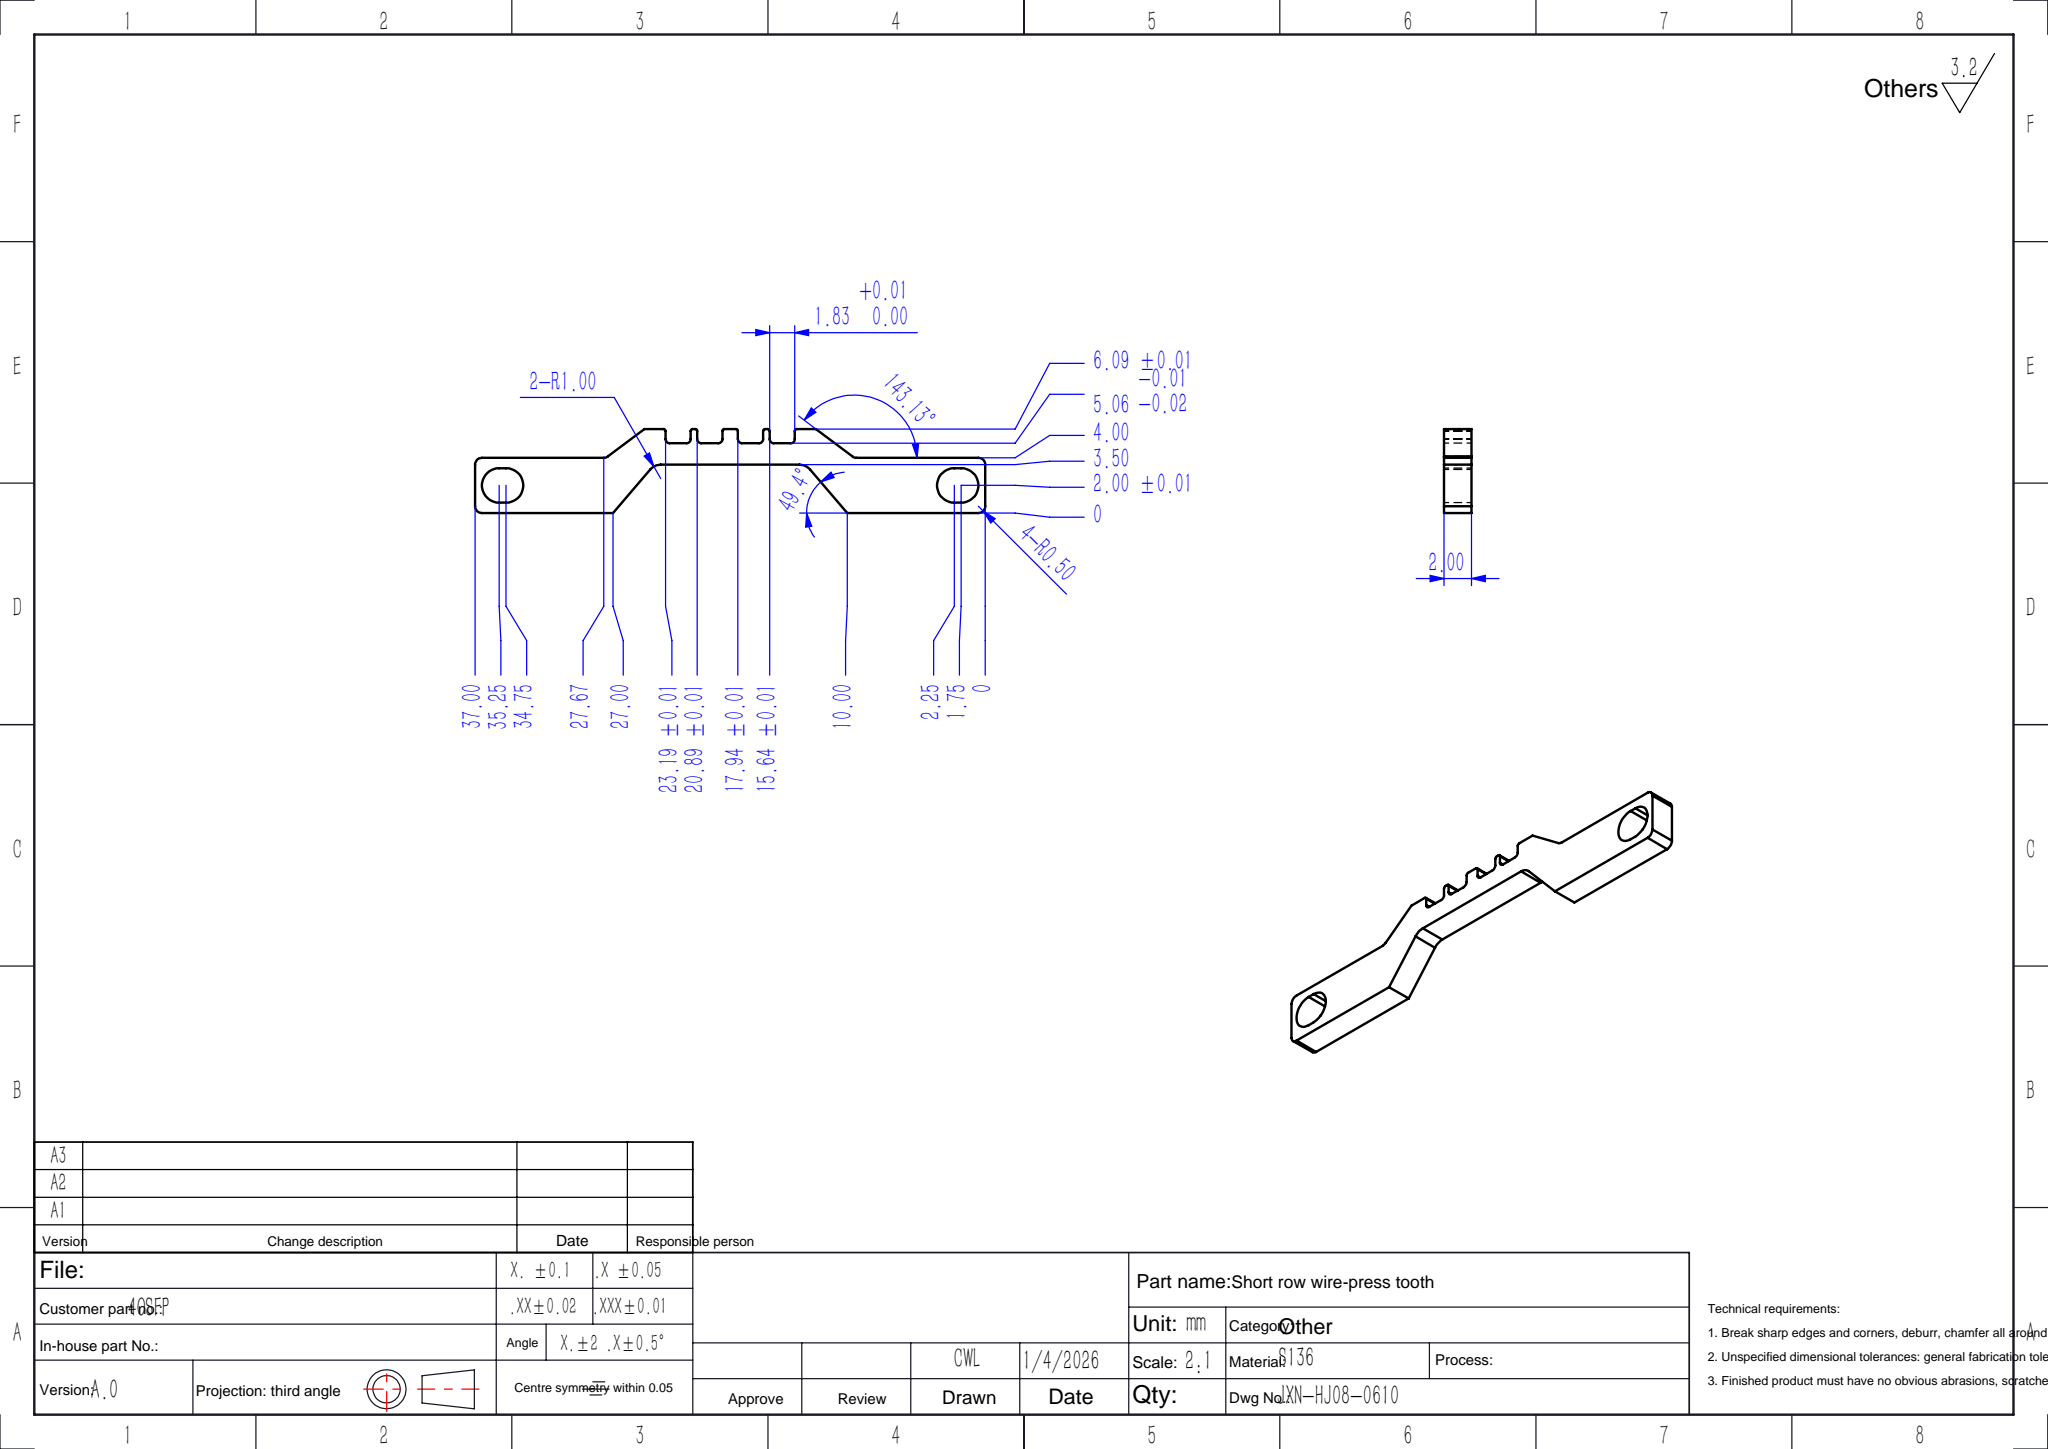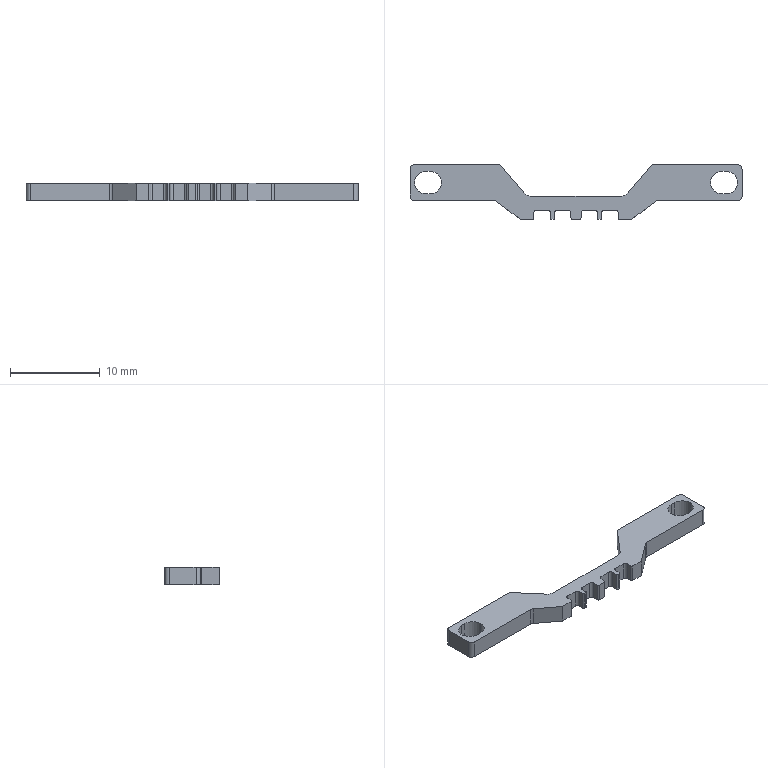Part | SolidWorks | features ICE 5, Fillet 2, Chamfer 1, Extrusion 1 | 1 solid | 64 faces | box 37 x 6.09 x 2 mm | volume 221.807 mm3 | plane 34 | cylinder 30 | commonest cylinder face diameters 0.3 x8 0.6 x8 1 x6 2.5 x6 2 x2